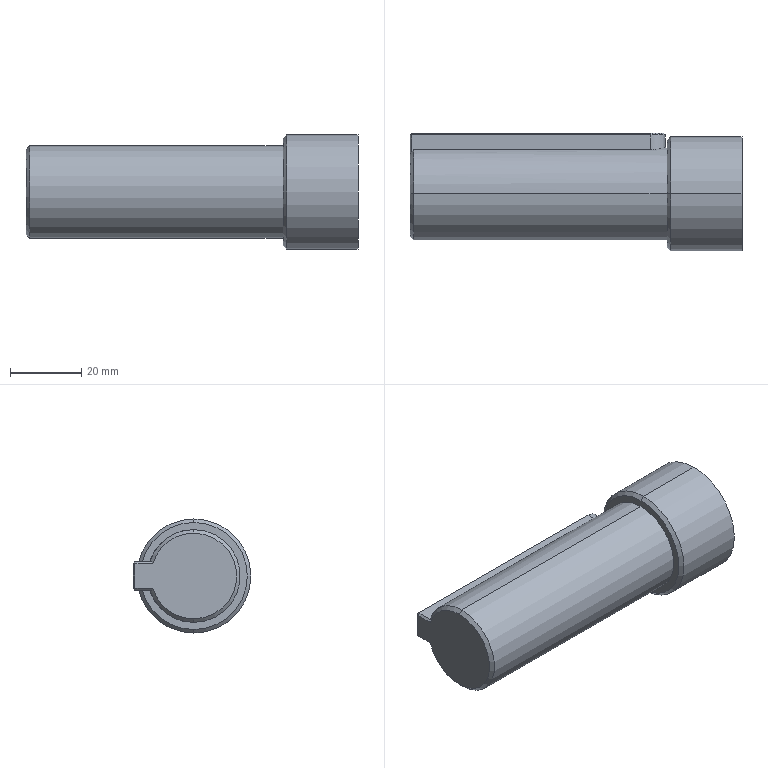Part | SolidWorks | features BaseBody 1 | 1 solid | 24 faces | box 93 x 33 x 32 mm | volume 57387 mm3 | plane 13 | cone 6 | cylinder 5 | commonest cylinder face diameters 26 x2 32 x2 8 x1
STEP:
#1=CARTESIAN_POINT('',(-3.357,18.855,4.));
#2=VERTEX_POINT('',#1);
#3=CARTESIAN_POINT('',(-3.357,6.485,13.));
#4=VERTEX_POINT('',#3);
#5=CARTESIAN_POINT('',(-3.357,6.485,0.));
#6=DIRECTION('',(1.,0.,0.));
#7=DIRECTION('',(0.,0.,-1.));
#8=AXIS2_PLACEMENT_3D('',#5,#6,#7);
#9=CIRCLE('',#8,13.);
#10=EDGE_CURVE('',#2,#4,#9,.T.);
#11=ORIENTED_EDGE('',*,*,#10,.T.);
#12=CARTESIAN_POINT('',(67.643,6.485,13.));
#13=VERTEX_POINT('',#12);
#14=CARTESIAN_POINT('',(31.643,6.485,13.));
#15=DIRECTION('',(1.,0.,0.));
#16=VECTOR('',#15,1000.);
#17=LINE('',#14,#16);
#18=EDGE_CURVE('',#4,#13,#17,.T.);
#19=ORIENTED_EDGE('',*,*,#18,.T.);
#20=CARTESIAN_POINT('',(67.643,6.485,-13.));
#21=VERTEX_POINT('',#20);
#22=CARTESIAN_POINT('',(67.643,6.485,0.));
#23=DIRECTION('',(-1.,0.,0.));
#24=DIRECTION('',(0.,0.,-1.));
#25=AXIS2_PLACEMENT_3D('',#22,#23,#24);
#26=CIRCLE('',#25,13.);
#27=EDGE_CURVE('',#13,#21,#26,.T.);
#28=ORIENTED_EDGE('',*,*,#27,.T.);
#29=CARTESIAN_POINT('',(-3.357,6.485,-13.));
#30=VERTEX_POINT('',#29);
#31=CARTESIAN_POINT('',(31.643,6.485,-13.));
#32=DIRECTION('',(1.,0.,0.));
#33=VECTOR('',#32,1000.);
#34=LINE('',#31,#33);
#35=EDGE_CURVE('',#30,#21,#34,.T.);
#36=ORIENTED_EDGE('',*,*,#35,.F.);
#37=CARTESIAN_POINT('',(-3.357,18.855,-4.));
#38=VERTEX_POINT('',#37);
#39=CARTESIAN_POINT('',(-3.357,6.485,0.));
#40=DIRECTION('',(1.,0.,0.));
#41=DIRECTION('',(0.,0.,-1.));
#42=AXIS2_PLACEMENT_3D('',#39,#40,#41);
#43=CIRCLE('',#42,13.);
#44=EDGE_CURVE('',#30,#38,#43,.T.);
#45=ORIENTED_EDGE('',*,*,#44,.T.);
#46=CARTESIAN_POINT('',(63.143,18.855,-4.));
#47=VERTEX_POINT('',#46);
#48=CARTESIAN_POINT('',(31.643,18.855,-4.));
#49=DIRECTION('',(1.,0.,0.));
#50=VECTOR('',#49,1000.);
#51=LINE('',#48,#50);
#52=EDGE_CURVE('',#38,#47,#51,.T.);
#53=ORIENTED_EDGE('',*,*,#52,.T.);
#54=CARTESIAN_POINT('',(63.143,18.855,4.));
#55=VERTEX_POINT('',#54);
#56=CARTESIAN_POINT('',(63.143,18.855,-4.));
#57=CARTESIAN_POINT('',(63.408,18.855,-4.));
#58=CARTESIAN_POINT('',(63.67,18.863,-3.974));
#59=CARTESIAN_POINT('',(64.183,18.896,-3.871));
#60=CARTESIAN_POINT('',(64.438,18.92,-3.794));
#61=CARTESIAN_POINT('',(64.921,18.98,-3.592));
#62=CARTESIAN_POINT('',(65.15,19.015,-3.469));
#63=CARTESIAN_POINT('',(65.584,19.092,-3.179));
#64=CARTESIAN_POINT('',(65.788,19.133,-3.012));
#65=CARTESIAN_POINT('',(66.154,19.215,-2.645));
#66=CARTESIAN_POINT('',(66.319,19.255,-2.445));
#67=CARTESIAN_POINT('',(66.612,19.331,-2.009));
#68=CARTESIAN_POINT('',(66.735,19.365,-1.779));
#69=CARTESIAN_POINT('',(66.935,19.423,-1.298));
#70=CARTESIAN_POINT('',(67.013,19.446,-1.044));
#71=CARTESIAN_POINT('',(67.116,19.477,-0.5272));
#72=CARTESIAN_POINT('',(67.142,19.485,-0.2667));
#73=CARTESIAN_POINT('',(67.143,19.486,0.2586));
#74=CARTESIAN_POINT('',(67.117,19.477,0.5255));
#75=CARTESIAN_POINT('',(67.014,19.446,1.04));
#76=CARTESIAN_POINT('',(66.938,19.424,1.29));
#77=CARTESIAN_POINT('',(66.736,19.366,1.776));
#78=CARTESIAN_POINT('',(66.612,19.331,2.008));
#79=CARTESIAN_POINT('',(66.323,19.256,2.44));
#80=CARTESIAN_POINT('',(66.156,19.215,2.643));
#81=CARTESIAN_POINT('',(65.787,19.133,3.012));
#82=CARTESIAN_POINT('',(65.587,19.092,3.177));
#83=CARTESIAN_POINT('',(65.156,19.016,3.466));
#84=CARTESIAN_POINT('',(64.922,18.98,3.592));
#85=CARTESIAN_POINT('',(64.44,18.92,3.793));
#86=CARTESIAN_POINT('',(64.191,18.896,3.869));
#87=CARTESIAN_POINT('',(63.674,18.863,3.973));
#88=CARTESIAN_POINT('',(63.408,18.855,4.));
#89=CARTESIAN_POINT('',(63.143,18.855,4.));
#90=B_SPLINE_CURVE_WITH_KNOTS('',3,(#56,#57,#58,#59,#60,#61,#62,#63,#64,#65,#66,#67,#68,#69,#70,#71,#72,#73,#74,#75,#76,#77,#78,#79,#80,#81,#82,#83,#84,#85,#86,#87,#88,#89),.UNSPECIFIED.,.F.,.F.,(4,2,2,2,2,2,2,2,2,2,2,2,2,2,2,2,4),(0.,0.0007861,0.001572,0.002358,0.003144,0.003931,0.004717,0.005503,0.006289,0.007075,0.007861,0.008647,0.009433,0.01022,0.01101,0.01179,0.01258),.UNSPECIFIED.);
#91=EDGE_CURVE('',#47,#55,#90,.T.);
#92=ORIENTED_EDGE('',*,*,#91,.T.);
#93=CARTESIAN_POINT('',(31.643,18.855,4.));
#94=DIRECTION('',(-1.,0.,0.));
#95=VECTOR('',#94,1000.);
#96=LINE('',#93,#95);
#97=EDGE_CURVE('',#55,#2,#96,.T.);
#98=ORIENTED_EDGE('',*,*,#97,.T.);
#99=EDGE_LOOP('',(#11,#19,#28,#36,#45,#53,#92,#98));
#100=FACE_OUTER_BOUND('',#99,.T.);
#101=CARTESIAN_POINT('',(31.643,6.485,0.));
#102=DIRECTION('',(1.,0.,0.));
#103=DIRECTION('',(0.,0.,-1.));
#104=AXIS2_PLACEMENT_3D('',#101,#102,#103);
#105=CYLINDRICAL_SURFACE('',#104,13.);
#106=ADVANCED_FACE('',(#100),#105,.T.);
#107=CARTESIAN_POINT('',(-4.357,17.964,3.5));
#108=VERTEX_POINT('',#107);
#109=CARTESIAN_POINT('',(-4.357,6.485,12.));
#110=VERTEX_POINT('',#109);
#111=CARTESIAN_POINT('',(-4.357,6.485,0.));
#112=DIRECTION('',(1.,0.,0.));
#113=DIRECTION('',(0.,0.,-1.));
#114=AXIS2_PLACEMENT_3D('',#111,#112,#113);
#115=CIRCLE('',#114,12.);
#116=EDGE_CURVE('',#108,#110,#115,.T.);
#117=ORIENTED_EDGE('',*,*,#116,.T.);
#118=CARTESIAN_POINT('',(-3.357,6.485,13.));
#119=DIRECTION('',(0.7071,0.,0.7071));
#120=VECTOR('',#119,1000.);
#121=LINE('',#118,#120);
#122=EDGE_CURVE('',#110,#4,#121,.T.);
#123=ORIENTED_EDGE('',*,*,#122,.T.);
#124=ORIENTED_EDGE('',*,*,#10,.F.);
#125=CARTESIAN_POINT('',(-3.857,18.328,4.));
#126=VERTEX_POINT('',#125);
#127=CARTESIAN_POINT('',(-3.857,18.328,4.));
#128=CARTESIAN_POINT('',(-3.691,18.504,4.));
#129=CARTESIAN_POINT('',(-3.524,18.679,4.));
#130=CARTESIAN_POINT('',(-3.357,18.855,4.));
#131=B_SPLINE_CURVE_WITH_KNOTS('',3,(#127,#128,#129,#130),.UNSPECIFIED.,.F.,.F.,(4,4),(0.,0.0007262),.UNSPECIFIED.);
#132=EDGE_CURVE('',#126,#2,#131,.T.);
#133=ORIENTED_EDGE('',*,*,#132,.F.);
#134=CARTESIAN_POINT('',(-3.857,18.328,4.));
#135=CARTESIAN_POINT('',(-4.025,18.208,3.833));
#136=CARTESIAN_POINT('',(-4.191,18.087,3.666));
#137=CARTESIAN_POINT('',(-4.357,17.964,3.5));
#138=B_SPLINE_CURVE_WITH_KNOTS('',3,(#134,#135,#136,#137),.UNSPECIFIED.,.F.,.F.,(4,4),(0.,0.0007955),.UNSPECIFIED.);
#139=EDGE_CURVE('',#126,#108,#138,.T.);
#140=ORIENTED_EDGE('',*,*,#139,.T.);
#141=EDGE_LOOP('',(#117,#123,#124,#133,#140));
#142=FACE_OUTER_BOUND('',#141,.T.);
#143=CARTESIAN_POINT('',(-3.357,6.485,0.));
#144=DIRECTION('',(1.,0.,0.));
#145=DIRECTION('',(0.,0.,-1.));
#146=AXIS2_PLACEMENT_3D('',#143,#144,#145);
#147=CONICAL_SURFACE('',#146,13.,0.7854);
#148=ADVANCED_FACE('',(#142),#147,.T.);
#149=ORIENTED_EDGE('',*,*,#122,.F.);
#150=CARTESIAN_POINT('',(-4.357,6.485,-12.));
#151=VERTEX_POINT('',#150);
#152=CARTESIAN_POINT('',(-4.357,6.485,0.));
#153=DIRECTION('',(1.,0.,0.));
#154=DIRECTION('',(0.,0.,-1.));
#155=AXIS2_PLACEMENT_3D('',#152,#153,#154);
#156=CIRCLE('',#155,12.);
#157=EDGE_CURVE('',#110,#151,#156,.T.);
#158=ORIENTED_EDGE('',*,*,#157,.T.);
#159=CARTESIAN_POINT('',(-3.357,6.485,-13.));
#160=DIRECTION('',(0.7071,0.,-0.7071));
#161=VECTOR('',#160,1000.);
#162=LINE('',#159,#161);
#163=EDGE_CURVE('',#151,#30,#162,.T.);
#164=ORIENTED_EDGE('',*,*,#163,.T.);
#165=CARTESIAN_POINT('',(-3.357,6.485,0.));
#166=DIRECTION('',(1.,0.,0.));
#167=DIRECTION('',(0.,0.,-1.));
#168=AXIS2_PLACEMENT_3D('',#165,#166,#167);
#169=CIRCLE('',#168,13.);
#170=EDGE_CURVE('',#4,#30,#169,.T.);
#171=ORIENTED_EDGE('',*,*,#170,.F.);
#172=EDGE_LOOP('',(#149,#158,#164,#171));
#173=FACE_OUTER_BOUND('',#172,.T.);
#174=CARTESIAN_POINT('',(-3.357,6.485,0.));
#175=DIRECTION('',(1.,0.,0.));
#176=DIRECTION('',(0.,0.,-1.));
#177=AXIS2_PLACEMENT_3D('',#174,#175,#176);
#178=CONICAL_SURFACE('',#177,13.,0.7854);
#179=ADVANCED_FACE('',(#173),#178,.T.);
#180=CARTESIAN_POINT('',(67.643,6.485,15.));
#181=VERTEX_POINT('',#180);
#182=CARTESIAN_POINT('',(67.643,6.485,-15.));
#183=VERTEX_POINT('',#182);
#184=CARTESIAN_POINT('',(67.643,6.485,0.));
#185=DIRECTION('',(-1.,0.,0.));
#186=DIRECTION('',(0.,0.,-1.));
#187=AXIS2_PLACEMENT_3D('',#184,#185,#186);
#188=CIRCLE('',#187,15.);
#189=EDGE_CURVE('',#181,#183,#188,.T.);
#190=ORIENTED_EDGE('',*,*,#189,.F.);
#191=CARTESIAN_POINT('',(68.643,6.485,16.));
#192=VERTEX_POINT('',#191);
#193=CARTESIAN_POINT('',(68.643,6.485,16.));
#194=DIRECTION('',(0.7071,0.,0.7071));
#195=VECTOR('',#194,1000.);
#196=LINE('',#193,#195);
#197=EDGE_CURVE('',#181,#192,#196,.T.);
#198=ORIENTED_EDGE('',*,*,#197,.T.);
#199=CARTESIAN_POINT('',(68.643,6.485,-16.));
#200=VERTEX_POINT('',#199);
#201=CARTESIAN_POINT('',(68.643,6.485,0.));
#202=DIRECTION('',(-1.,0.,0.));
#203=DIRECTION('',(0.,-1.,0.));
#204=AXIS2_PLACEMENT_3D('',#201,#202,#203);
#205=CIRCLE('',#204,16.);
#206=EDGE_CURVE('',#192,#200,#205,.T.);
#207=ORIENTED_EDGE('',*,*,#206,.T.);
#208=CARTESIAN_POINT('',(68.643,6.485,-16.));
#209=DIRECTION('',(0.7071,0.,-0.7071));
#210=VECTOR('',#209,1000.);
#211=LINE('',#208,#210);
#212=EDGE_CURVE('',#183,#200,#211,.T.);
#213=ORIENTED_EDGE('',*,*,#212,.F.);
#214=EDGE_LOOP('',(#190,#198,#207,#213));
#215=FACE_OUTER_BOUND('',#214,.T.);
#216=CARTESIAN_POINT('',(68.643,6.485,0.));
#217=DIRECTION('',(1.,0.,0.));
#218=DIRECTION('',(0.,0.,-1.));
#219=AXIS2_PLACEMENT_3D('',#216,#217,#218);
#220=CONICAL_SURFACE('',#219,16.,0.7854);
#221=ADVANCED_FACE('',(#215),#220,.T.);
#222=ORIENTED_EDGE('',*,*,#206,.F.);
#223=CARTESIAN_POINT('',(88.643,6.485,16.));
#224=VERTEX_POINT('',#223);
#225=CARTESIAN_POINT('',(78.143,6.485,16.));
#226=DIRECTION('',(1.,0.,0.));
#227=VECTOR('',#226,1000.);
#228=LINE('',#225,#227);
#229=EDGE_CURVE('',#192,#224,#228,.T.);
#230=ORIENTED_EDGE('',*,*,#229,.T.);
#231=CARTESIAN_POINT('',(88.643,6.485,-16.));
#232=VERTEX_POINT('',#231);
#233=CARTESIAN_POINT('',(88.643,6.485,0.));
#234=DIRECTION('',(-1.,0.,0.));
#235=DIRECTION('',(0.,0.,-1.));
#236=AXIS2_PLACEMENT_3D('',#233,#234,#235);
#237=CIRCLE('',#236,16.);
#238=EDGE_CURVE('',#224,#232,#237,.T.);
#239=ORIENTED_EDGE('',*,*,#238,.T.);
#240=CARTESIAN_POINT('',(78.143,6.485,-16.));
#241=DIRECTION('',(1.,0.,0.));
#242=VECTOR('',#241,1000.);
#243=LINE('',#240,#242);
#244=EDGE_CURVE('',#200,#232,#243,.T.);
#245=ORIENTED_EDGE('',*,*,#244,.F.);
#246=EDGE_LOOP('',(#222,#230,#239,#245));
#247=FACE_OUTER_BOUND('',#246,.T.);
#248=CARTESIAN_POINT('',(78.143,6.485,0.));
#249=DIRECTION('',(1.,0.,0.));
#250=DIRECTION('',(0.,0.,-1.));
#251=AXIS2_PLACEMENT_3D('',#248,#249,#250);
#252=CYLINDRICAL_SURFACE('',#251,16.);
#253=ADVANCED_FACE('',(#247),#252,.T.);
#254=ORIENTED_EDGE('',*,*,#18,.F.);
#255=ORIENTED_EDGE('',*,*,#170,.T.);
#256=ORIENTED_EDGE('',*,*,#35,.T.);
#257=CARTESIAN_POINT('',(67.643,6.485,0.));
#258=DIRECTION('',(-1.,0.,0.));
#259=DIRECTION('',(0.,0.,-1.));
#260=AXIS2_PLACEMENT_3D('',#257,#258,#259);
#261=CIRCLE('',#260,13.);
#262=EDGE_CURVE('',#21,#13,#261,.T.);
#263=ORIENTED_EDGE('',*,*,#262,.T.);
#264=EDGE_LOOP('',(#254,#255,#256,#263));
#265=FACE_OUTER_BOUND('',#264,.T.);
#266=CARTESIAN_POINT('',(31.643,6.485,0.));
#267=DIRECTION('',(1.,0.,0.));
#268=DIRECTION('',(0.,0.,-1.));
#269=AXIS2_PLACEMENT_3D('',#266,#267,#268);
#270=CYLINDRICAL_SURFACE('',#269,13.);
#271=ADVANCED_FACE('',(#265),#270,.T.);
#272=ORIENTED_EDGE('',*,*,#262,.F.);
#273=ORIENTED_EDGE('',*,*,#27,.F.);
#274=EDGE_LOOP('',(#272,#273));
#275=FACE_BOUND('',#274,.T.);
#276=CARTESIAN_POINT('',(67.643,6.485,0.));
#277=DIRECTION('',(-1.,0.,0.));
#278=DIRECTION('',(0.,0.,-1.));
#279=AXIS2_PLACEMENT_3D('',#276,#277,#278);
#280=CIRCLE('',#279,15.);
#281=EDGE_CURVE('',#183,#181,#280,.T.);
#282=ORIENTED_EDGE('',*,*,#281,.T.);
#283=ORIENTED_EDGE('',*,*,#189,.T.);
#284=EDGE_LOOP('',(#282,#283));
#285=FACE_OUTER_BOUND('',#284,.T.);
#286=CARTESIAN_POINT('',(67.643,20.985,0.));
#287=DIRECTION('',(-1.,0.,0.));
#288=DIRECTION('',(0.,0.,1.));
#289=AXIS2_PLACEMENT_3D('',#286,#287,#288);
#290=PLANE('',#289);
#291=ADVANCED_FACE('',(#275,#285),#290,.T.);
#292=CARTESIAN_POINT('',(63.143,22.985,4.));
#293=VERTEX_POINT('',#292);
#294=CARTESIAN_POINT('',(63.143,19.485,4.));
#295=DIRECTION('',(0.,1.,0.));
#296=VECTOR('',#295,1000.);
#297=LINE('',#294,#296);
#298=EDGE_CURVE('',#55,#293,#297,.T.);
#299=ORIENTED_EDGE('',*,*,#298,.T.);
#300=CARTESIAN_POINT('',(-3.857,22.985,4.));
#301=VERTEX_POINT('',#300);
#302=CARTESIAN_POINT('',(63.143,22.985,4.));
#303=DIRECTION('',(-1.,0.,0.));
#304=VECTOR('',#303,1000.);
#305=LINE('',#302,#304);
#306=EDGE_CURVE('',#293,#301,#305,.T.);
#307=ORIENTED_EDGE('',*,*,#306,.T.);
#308=CARTESIAN_POINT('',(-3.857,19.485,4.));
#309=DIRECTION('',(0.,-1.,0.));
#310=VECTOR('',#309,1000.);
#311=LINE('',#308,#310);
#312=EDGE_CURVE('',#301,#126,#311,.T.);
#313=ORIENTED_EDGE('',*,*,#312,.T.);
#314=ORIENTED_EDGE('',*,*,#132,.T.);
#315=ORIENTED_EDGE('',*,*,#97,.F.);
#316=EDGE_LOOP('',(#299,#307,#313,#314,#315));
#317=FACE_OUTER_BOUND('',#316,.T.);
#318=CARTESIAN_POINT('',(63.143,19.485,4.));
#319=DIRECTION('',(0.,0.,1.));
#320=DIRECTION('',(1.,0.,0.));
#321=AXIS2_PLACEMENT_3D('',#318,#319,#320);
#322=PLANE('',#321);
#323=ADVANCED_FACE('',(#317),#322,.T.);
#324=ORIENTED_EDGE('',*,*,#91,.F.);
#325=CARTESIAN_POINT('',(63.143,22.985,-4.));
#326=VERTEX_POINT('',#325);
#327=CARTESIAN_POINT('',(63.143,19.485,-4.));
#328=DIRECTION('',(0.,1.,0.));
#329=VECTOR('',#328,1000.);
#330=LINE('',#327,#329);
#331=EDGE_CURVE('',#47,#326,#330,.T.);
#332=ORIENTED_EDGE('',*,*,#331,.T.);
#333=CARTESIAN_POINT('',(63.143,22.985,0.));
#334=DIRECTION('',(0.,-1.,0.));
#335=DIRECTION('',(0.,0.,1.));
#336=AXIS2_PLACEMENT_3D('',#333,#334,#335);
#337=CIRCLE('',#336,4.);
#338=EDGE_CURVE('',#326,#293,#337,.T.);
#339=ORIENTED_EDGE('',*,*,#338,.T.);
#340=ORIENTED_EDGE('',*,*,#298,.F.);
#341=EDGE_LOOP('',(#324,#332,#339,#340));
#342=FACE_OUTER_BOUND('',#341,.T.);
#343=CARTESIAN_POINT('',(63.143,19.485,0.));
#344=DIRECTION('',(0.,1.,0.));
#345=DIRECTION('',(0.,0.,1.));
#346=AXIS2_PLACEMENT_3D('',#343,#344,#345);
#347=CYLINDRICAL_SURFACE('',#346,4.);
#348=ADVANCED_FACE('',(#342),#347,.T.);
#349=ORIENTED_EDGE('',*,*,#52,.F.);
#350=CARTESIAN_POINT('',(-3.857,18.328,-4.));
#351=VERTEX_POINT('',#350);
#352=CARTESIAN_POINT('',(-3.357,18.855,-4.));
#353=CARTESIAN_POINT('',(-3.524,18.679,-4.));
#354=CARTESIAN_POINT('',(-3.691,18.504,-4.));
#355=CARTESIAN_POINT('',(-3.857,18.328,-4.));
#356=B_SPLINE_CURVE_WITH_KNOTS('',3,(#352,#353,#354,#355),.UNSPECIFIED.,.F.,.F.,(4,4),(0.,0.0007262),.UNSPECIFIED.);
#357=EDGE_CURVE('',#38,#351,#356,.T.);
#358=ORIENTED_EDGE('',*,*,#357,.T.);
#359=CARTESIAN_POINT('',(-3.857,22.985,-4.));
#360=VERTEX_POINT('',#359);
#361=CARTESIAN_POINT('',(-3.857,19.485,-4.));
#362=DIRECTION('',(0.,1.,0.));
#363=VECTOR('',#362,1000.);
#364=LINE('',#361,#363);
#365=EDGE_CURVE('',#351,#360,#364,.T.);
#366=ORIENTED_EDGE('',*,*,#365,.T.);
#367=CARTESIAN_POINT('',(-4.357,22.985,-4.));
#368=DIRECTION('',(1.,0.,0.));
#369=VECTOR('',#368,1000.);
#370=LINE('',#367,#369);
#371=EDGE_CURVE('',#360,#326,#370,.T.);
#372=ORIENTED_EDGE('',*,*,#371,.T.);
#373=ORIENTED_EDGE('',*,*,#331,.F.);
#374=EDGE_LOOP('',(#349,#358,#366,#372,#373));
#375=FACE_OUTER_BOUND('',#374,.T.);
#376=CARTESIAN_POINT('',(-4.357,19.485,-4.));
#377=DIRECTION('',(0.,0.,-1.));
#378=DIRECTION('',(-1.,0.,0.));
#379=AXIS2_PLACEMENT_3D('',#376,#377,#378);
#380=PLANE('',#379);
#381=ADVANCED_FACE('',(#375),#380,.T.);
#382=ORIENTED_EDGE('',*,*,#163,.F.);
#383=CARTESIAN_POINT('',(-4.357,17.964,-3.5));
#384=VERTEX_POINT('',#383);
#385=CARTESIAN_POINT('',(-4.357,6.485,0.));
#386=DIRECTION('',(1.,0.,0.));
#387=DIRECTION('',(0.,0.,-1.));
#388=AXIS2_PLACEMENT_3D('',#385,#386,#387);
#389=CIRCLE('',#388,12.);
#390=EDGE_CURVE('',#151,#384,#389,.T.);
#391=ORIENTED_EDGE('',*,*,#390,.T.);
#392=CARTESIAN_POINT('',(-4.357,17.964,-3.5));
#393=CARTESIAN_POINT('',(-4.191,18.087,-3.666));
#394=CARTESIAN_POINT('',(-4.025,18.208,-3.833));
#395=CARTESIAN_POINT('',(-3.857,18.328,-4.));
#396=B_SPLINE_CURVE_WITH_KNOTS('',3,(#392,#393,#394,#395),.UNSPECIFIED.,.F.,.F.,(4,4),(0.,0.0007955),.UNSPECIFIED.);
#397=EDGE_CURVE('',#384,#351,#396,.T.);
#398=ORIENTED_EDGE('',*,*,#397,.T.);
#399=ORIENTED_EDGE('',*,*,#357,.F.);
#400=ORIENTED_EDGE('',*,*,#44,.F.);
#401=EDGE_LOOP('',(#382,#391,#398,#399,#400));
#402=FACE_OUTER_BOUND('',#401,.T.);
#403=CARTESIAN_POINT('',(-3.357,6.485,0.));
#404=DIRECTION('',(1.,0.,0.));
#405=DIRECTION('',(0.,0.,-1.));
#406=AXIS2_PLACEMENT_3D('',#403,#404,#405);
#407=CONICAL_SURFACE('',#406,13.,0.7854);
#408=ADVANCED_FACE('',(#402),#407,.T.);
#409=ORIENTED_EDGE('',*,*,#197,.F.);
#410=ORIENTED_EDGE('',*,*,#281,.F.);
#411=ORIENTED_EDGE('',*,*,#212,.T.);
#412=CARTESIAN_POINT('',(68.643,6.485,0.));
#413=DIRECTION('',(-1.,0.,0.));
#414=DIRECTION('',(0.,-1.,0.));
#415=AXIS2_PLACEMENT_3D('',#412,#413,#414);
#416=CIRCLE('',#415,16.);
#417=EDGE_CURVE('',#200,#192,#416,.T.);
#418=ORIENTED_EDGE('',*,*,#417,.T.);
#419=EDGE_LOOP('',(#409,#410,#411,#418));
#420=FACE_OUTER_BOUND('',#419,.T.);
#421=CARTESIAN_POINT('',(68.643,6.485,0.));
#422=DIRECTION('',(1.,0.,0.));
#423=DIRECTION('',(0.,0.,-1.));
#424=AXIS2_PLACEMENT_3D('',#421,#422,#423);
#425=CONICAL_SURFACE('',#424,16.,0.7854);
#426=ADVANCED_FACE('',(#420),#425,.T.);
#427=CARTESIAN_POINT('',(63.143,23.485,3.5));
#428=VERTEX_POINT('',#427);
#429=CARTESIAN_POINT('',(63.143,23.235,3.75));
#430=DIRECTION('',(0.,0.7071,-0.7071));
#431=VECTOR('',#430,1000.);
#432=LINE('',#429,#431);
#433=EDGE_CURVE('',#293,#428,#432,.T.);
#434=ORIENTED_EDGE('',*,*,#433,.T.);
#435=CARTESIAN_POINT('',(-3.857,23.485,3.5));
#436=VERTEX_POINT('',#435);
#437=CARTESIAN_POINT('',(46.856,23.485,3.5));
#438=DIRECTION('',(-1.,0.,0.));
#439=VECTOR('',#438,1000.);
#440=LINE('',#437,#439);
#441=EDGE_CURVE('',#428,#436,#440,.T.);
#442=ORIENTED_EDGE('',*,*,#441,.T.);
#443=CARTESIAN_POINT('',(-3.857,23.235,3.75));
#444=DIRECTION('',(0.,-0.7071,0.7071));
#445=VECTOR('',#444,1000.);
#446=LINE('',#443,#445);
#447=EDGE_CURVE('',#436,#301,#446,.T.);
#448=ORIENTED_EDGE('',*,*,#447,.T.);
#449=ORIENTED_EDGE('',*,*,#306,.F.);
#450=EDGE_LOOP('',(#434,#442,#448,#449));
#451=FACE_OUTER_BOUND('',#450,.T.);
#452=CARTESIAN_POINT('',(46.856,23.235,3.75));
#453=DIRECTION('',(0.,0.7071,0.7071));
#454=DIRECTION('',(0.,-0.7071,0.7071));
#455=AXIS2_PLACEMENT_3D('',#452,#453,#454);
#456=PLANE('',#455);
#457=ADVANCED_FACE('',(#451),#456,.T.);
#458=CARTESIAN_POINT('',(-4.357,22.985,3.5));
#459=VERTEX_POINT('',#458);
#460=CARTESIAN_POINT('',(-4.107,22.985,3.75));
#461=DIRECTION('',(-0.7071,0.,-0.7071));
#462=VECTOR('',#461,1000.);
#463=LINE('',#460,#462);
#464=EDGE_CURVE('',#301,#459,#463,.T.);
#465=ORIENTED_EDGE('',*,*,#464,.T.);
#466=CARTESIAN_POINT('',(-4.357,16.235,3.5));
#467=DIRECTION('',(0.,-1.,0.));
#468=VECTOR('',#467,1000.);
#469=LINE('',#466,#468);
#470=EDGE_CURVE('',#459,#108,#469,.T.);
#471=ORIENTED_EDGE('',*,*,#470,.T.);
#472=ORIENTED_EDGE('',*,*,#139,.F.);
#473=ORIENTED_EDGE('',*,*,#312,.F.);
#474=EDGE_LOOP('',(#465,#471,#472,#473));
#475=FACE_OUTER_BOUND('',#474,.T.);
#476=CARTESIAN_POINT('',(-4.107,16.235,3.75));
#477=DIRECTION('',(-0.7071,0.,0.7071));
#478=DIRECTION('',(0.7071,0.,0.7071));
#479=AXIS2_PLACEMENT_3D('',#476,#477,#478);
#480=PLANE('',#479);
#481=ADVANCED_FACE('',(#475),#480,.T.);
#482=CARTESIAN_POINT('',(63.143,23.485,-3.5));
#483=VERTEX_POINT('',#482);
#484=CARTESIAN_POINT('',(63.143,-498973.015,-499000.));
#485=DIRECTION('',(0.,0.7071,0.7071));
#486=VECTOR('',#485,1000.);
#487=LINE('',#484,#486);
#488=EDGE_CURVE('',#326,#483,#487,.T.);
#489=ORIENTED_EDGE('',*,*,#488,.T.);
#490=CARTESIAN_POINT('',(63.143,23.485,0.));
#491=DIRECTION('',(0.,-1.,0.));
#492=DIRECTION('',(0.,0.,-1.));
#493=AXIS2_PLACEMENT_3D('',#490,#491,#492);
#494=CIRCLE('',#493,3.5);
#495=EDGE_CURVE('',#483,#428,#494,.T.);
#496=ORIENTED_EDGE('',*,*,#495,.T.);
#497=ORIENTED_EDGE('',*,*,#433,.F.);
#498=ORIENTED_EDGE('',*,*,#338,.F.);
#499=EDGE_LOOP('',(#489,#496,#497,#498));
#500=FACE_OUTER_BOUND('',#499,.T.);
#501=CARTESIAN_POINT('',(63.143,22.985,0.));
#502=DIRECTION('',(0.,-1.,0.));
#503=DIRECTION('',(0.,0.,-1.));
#504=AXIS2_PLACEMENT_3D('',#501,#502,#503);
#505=CONICAL_SURFACE('',#504,4.,0.7854);
#506=ADVANCED_FACE('',(#500),#505,.T.);
#507=CARTESIAN_POINT('',(-3.857,23.485,-3.5));
#508=VERTEX_POINT('',#507);
#509=CARTESIAN_POINT('',(-3.857,23.235,-3.75));
#510=DIRECTION('',(0.,0.7071,0.7071));
#511=VECTOR('',#510,1000.);
#512=LINE('',#509,#511);
#513=EDGE_CURVE('',#360,#508,#512,.T.);
#514=ORIENTED_EDGE('',*,*,#513,.T.);
#515=CARTESIAN_POINT('',(13.106,23.485,-3.5));
#516=DIRECTION('',(1.,0.,0.));
#517=VECTOR('',#516,1000.);
#518=LINE('',#515,#517);
#519=EDGE_CURVE('',#508,#483,#518,.T.);
#520=ORIENTED_EDGE('',*,*,#519,.T.);
#521=ORIENTED_EDGE('',*,*,#488,.F.);
#522=ORIENTED_EDGE('',*,*,#371,.F.);
#523=EDGE_LOOP('',(#514,#520,#521,#522));
#524=FACE_OUTER_BOUND('',#523,.T.);
#525=CARTESIAN_POINT('',(13.106,23.235,-3.75));
#526=DIRECTION('',(0.,0.7071,-0.7071));
#527=DIRECTION('',(0.,0.7071,0.7071));
#528=AXIS2_PLACEMENT_3D('',#525,#526,#527);
#529=PLANE('',#528);
#530=ADVANCED_FACE('',(#524),#529,.T.);
#531=CARTESIAN_POINT('',(-4.357,22.985,-3.5));
#532=VERTEX_POINT('',#531);
#533=CARTESIAN_POINT('',(-4.107,22.985,-3.75));
#534=DIRECTION('',(0.7071,0.,-0.7071));
#535=VECTOR('',#534,1000.);
#536=LINE('',#533,#535);
#537=EDGE_CURVE('',#532,#360,#536,.T.);
#538=ORIENTED_EDGE('',*,*,#537,.T.);
#539=ORIENTED_EDGE('',*,*,#365,.F.);
#540=ORIENTED_EDGE('',*,*,#397,.F.);
#541=CARTESIAN_POINT('',(-4.357,16.235,-3.5));
#542=DIRECTION('',(0.,1.,0.));
#543=VECTOR('',#542,1000.);
#544=LINE('',#541,#543);
#545=EDGE_CURVE('',#384,#532,#544,.T.);
#546=ORIENTED_EDGE('',*,*,#545,.T.);
#547=EDGE_LOOP('',(#538,#539,#540,#546));
#548=FACE_OUTER_BOUND('',#547,.T.);
#549=CARTESIAN_POINT('',(-4.107,16.235,-3.75));
#550=DIRECTION('',(-0.7071,0.,-0.7071));
#551=DIRECTION('',(-0.7071,0.,0.7071));
#552=AXIS2_PLACEMENT_3D('',#549,#550,#551);
#553=PLANE('',#552);
#554=ADVANCED_FACE('',(#548),#553,.T.);
#555=CARTESIAN_POINT('',(-4.357,22.985,0.));
#556=DIRECTION('',(0.,0.,-1.));
#557=VECTOR('',#556,1000.);
#558=LINE('',#555,#557);
#559=EDGE_CURVE('',#459,#532,#558,.T.);
#560=ORIENTED_EDGE('',*,*,#559,.T.);
#561=ORIENTED_EDGE('',*,*,#545,.F.);
#562=ORIENTED_EDGE('',*,*,#390,.F.);
#563=ORIENTED_EDGE('',*,*,#157,.F.);
#564=ORIENTED_EDGE('',*,*,#116,.F.);
#565=ORIENTED_EDGE('',*,*,#470,.F.);
#566=EDGE_LOOP('',(#560,#561,#562,#563,#564,#565));
#567=FACE_OUTER_BOUND('',#566,.T.);
#568=CARTESIAN_POINT('',(-4.357,12.985,0.));
#569=DIRECTION('',(-1.,0.,0.));
#570=DIRECTION('',(0.,0.,1.));
#571=AXIS2_PLACEMENT_3D('',#568,#569,#570);
#572=PLANE('',#571);
#573=ADVANCED_FACE('',(#567),#572,.T.);
#574=ORIENTED_EDGE('',*,*,#229,.F.);
#575=ORIENTED_EDGE('',*,*,#417,.F.);
#576=ORIENTED_EDGE('',*,*,#244,.T.);
#577=CARTESIAN_POINT('',(88.643,6.485,0.));
#578=DIRECTION('',(-1.,0.,0.));
#579=DIRECTION('',(0.,0.,-1.));
#580=AXIS2_PLACEMENT_3D('',#577,#578,#579);
#581=CIRCLE('',#580,16.);
#582=EDGE_CURVE('',#232,#224,#581,.T.);
#583=ORIENTED_EDGE('',*,*,#582,.T.);
#584=EDGE_LOOP('',(#574,#575,#576,#583));
#585=FACE_OUTER_BOUND('',#584,.T.);
#586=CARTESIAN_POINT('',(78.143,6.485,0.));
#587=DIRECTION('',(1.,0.,0.));
#588=DIRECTION('',(0.,0.,-1.));
#589=AXIS2_PLACEMENT_3D('',#586,#587,#588);
#590=CYLINDRICAL_SURFACE('',#589,16.);
#591=ADVANCED_FACE('',(#585),#590,.T.);
#592=ORIENTED_EDGE('',*,*,#441,.F.);
#593=ORIENTED_EDGE('',*,*,#495,.F.);
#594=ORIENTED_EDGE('',*,*,#519,.F.);
#595=CARTESIAN_POINT('',(-3.857,23.485,0.));
#596=DIRECTION('',(0.,0.,1.));
#597=VECTOR('',#596,1000.);
#598=LINE('',#595,#597);
#599=EDGE_CURVE('',#508,#436,#598,.T.);
#600=ORIENTED_EDGE('',*,*,#599,.T.);
#601=EDGE_LOOP('',(#592,#593,#594,#600));
#602=FACE_OUTER_BOUND('',#601,.T.);
#603=CARTESIAN_POINT('',(30.569,23.485,0.));
#604=DIRECTION('',(0.,1.,0.));
#605=DIRECTION('',(0.,0.,1.));
#606=AXIS2_PLACEMENT_3D('',#603,#604,#605);
#607=PLANE('',#606);
#608=ADVANCED_FACE('',(#602),#607,.T.);
#609=CARTESIAN_POINT('',(-4.232,23.11,3.5));
#610=DIRECTION('',(-0.7071,-0.7071,0.));
#611=VECTOR('',#610,1000.);
#612=LINE('',#609,#611);
#613=EDGE_CURVE('',#436,#459,#612,.T.);
#614=ORIENTED_EDGE('',*,*,#613,.T.);
#615=ORIENTED_EDGE('',*,*,#464,.F.);
#616=ORIENTED_EDGE('',*,*,#447,.F.);
#617=EDGE_LOOP('',(#614,#615,#616));
#618=FACE_OUTER_BOUND('',#617,.T.);
#619=CARTESIAN_POINT('',(-4.107,22.985,3.75));
#620=DIRECTION('',(-0.5774,0.5774,0.5774));
#621=DIRECTION('',(-0.7071,-0.7071,0.));
#622=AXIS2_PLACEMENT_3D('',#619,#620,#621);
#623=PLANE('',#622);
#624=ADVANCED_FACE('',(#618),#623,.T.);
#625=ORIENTED_EDGE('',*,*,#513,.F.);
#626=ORIENTED_EDGE('',*,*,#537,.F.);
#627=CARTESIAN_POINT('',(-4.357,22.985,-3.5));
#628=DIRECTION('',(0.7071,0.7071,0.));
#629=VECTOR('',#628,1000.);
#630=LINE('',#627,#629);
#631=EDGE_CURVE('',#532,#508,#630,.T.);
#632=ORIENTED_EDGE('',*,*,#631,.T.);
#633=EDGE_LOOP('',(#625,#626,#632));
#634=FACE_OUTER_BOUND('',#633,.T.);
#635=CARTESIAN_POINT('',(-4.107,22.985,-3.75));
#636=DIRECTION('',(-0.5774,0.5774,-0.5774));
#637=DIRECTION('',(0.,0.7071,0.7071));
#638=AXIS2_PLACEMENT_3D('',#635,#636,#637);
#639=PLANE('',#638);
#640=ADVANCED_FACE('',(#634),#639,.T.);
#641=ORIENTED_EDGE('',*,*,#613,.F.);
#642=ORIENTED_EDGE('',*,*,#599,.F.);
#643=ORIENTED_EDGE('',*,*,#631,.F.);
#644=ORIENTED_EDGE('',*,*,#559,.F.);
#645=EDGE_LOOP('',(#641,#642,#643,#644));
#646=FACE_OUTER_BOUND('',#645,.T.);
#647=CARTESIAN_POINT('',(-4.107,23.235,0.));
#648=DIRECTION('',(-0.7071,0.7071,0.));
#649=DIRECTION('',(-0.7071,-0.7071,0.));
#650=AXIS2_PLACEMENT_3D('',#647,#648,#649);
#651=PLANE('',#650);
#652=ADVANCED_FACE('',(#646),#651,.T.);
#653=ORIENTED_EDGE('',*,*,#582,.F.);
#654=ORIENTED_EDGE('',*,*,#238,.F.);
#655=EDGE_LOOP('',(#653,#654));
#656=FACE_OUTER_BOUND('',#655,.T.);
#657=CARTESIAN_POINT('',(88.643,14.485,0.));
#658=DIRECTION('',(1.,0.,0.));
#659=DIRECTION('',(0.,0.,-1.));
#660=AXIS2_PLACEMENT_3D('',#657,#658,#659);
#661=PLANE('',#660);
#662=ADVANCED_FACE('',(#656),#661,.T.);
#663=CLOSED_SHELL('',(#106,#148,#179,#221,#253,#271,#291,#323,#348,#381,#408,#426,#457,#481,#506,#530,#554,#573,#591,#608,#624,#640,#652,#662));
#664=MANIFOLD_SOLID_BREP('',#663);
#665=CARTESIAN_POINT('',(0.,0.,0.));
#666=DIRECTION('',(0.,0.,1.));
#667=DIRECTION('',(1.,0.,0.));
#668=AXIS2_PLACEMENT_3D('',#665,#666,#667);
#669=(LENGTH_UNIT()NAMED_UNIT(*)SI_UNIT(.MILLI.,.METRE.));
#670=UNCERTAINTY_MEASURE_WITH_UNIT(LENGTH_MEASURE(0.00001),#669,'','');
#671=(NAMED_UNIT(*)PLANE_ANGLE_UNIT()SI_UNIT($,.RADIAN.));
#672=(NAMED_UNIT(*)SI_UNIT($,.STERADIAN.)SOLID_ANGLE_UNIT());
#673=(GEOMETRIC_REPRESENTATION_CONTEXT(3)GLOBAL_UNCERTAINTY_ASSIGNED_CONTEXT((#670))GLOBAL_UNIT_ASSIGNED_CONTEXT((#669,#671,#672))REPRESENTATION_CONTEXT('',''));
#674=ADVANCED_BREP_SHAPE_REPRESENTATION('',(#664,#668),#673);